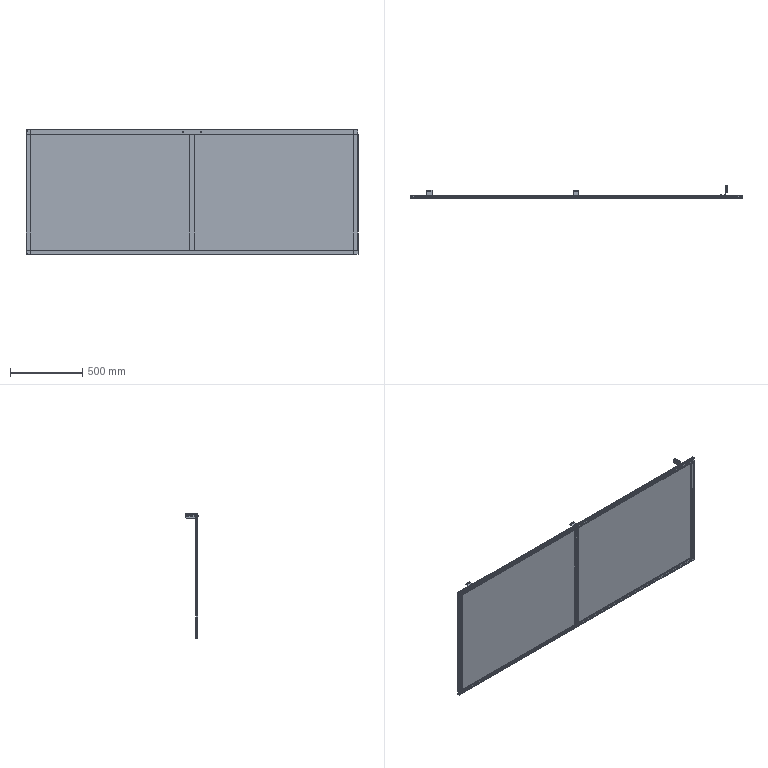Part | SolidWorks | features ReferencePattern 7, LocalLPattern 2 | 46 solids | 2030 faces | box 2296 x 92.007 x 864.302 mm | volume 10874128 mm3 | plane 1204 | cylinder 395 | spline 227 | cone 186 | torus 12 | sphere 6 | commonest cylinder face diameters 5 x67 11 x52 1 x42 4.5 x36 3.3 x24 6 x24